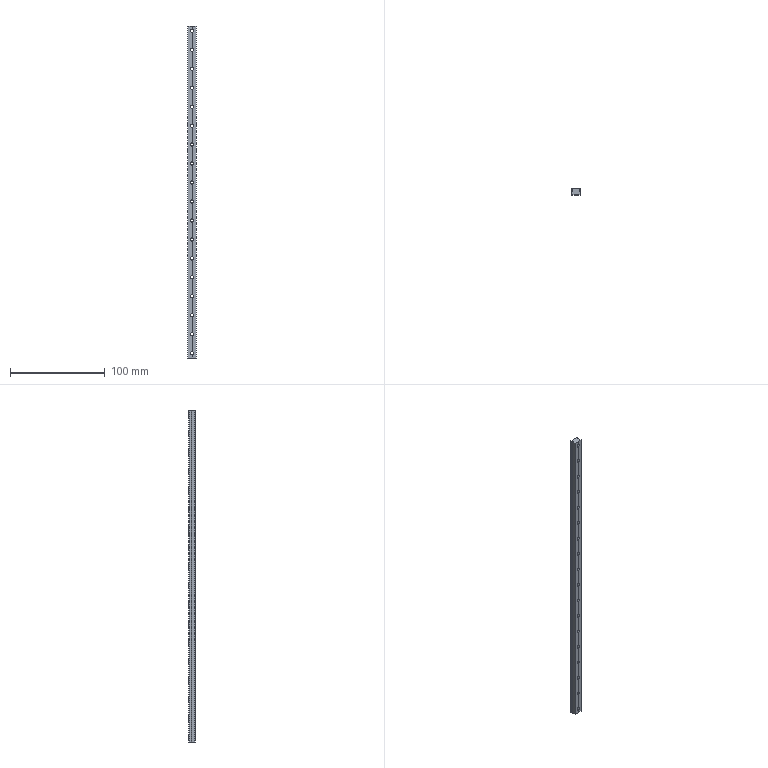Part | STEP file | MGN9 guide rail 1001 | 1 solid | 125 faces | box 9 x 6.5 x 350 mm | volume 17052 mm3 | cylinder 94 | plane 31 | commonest cylinder face diameters 6 x36 3.4 x26 0.6 x19 3.5 x10 2 x3